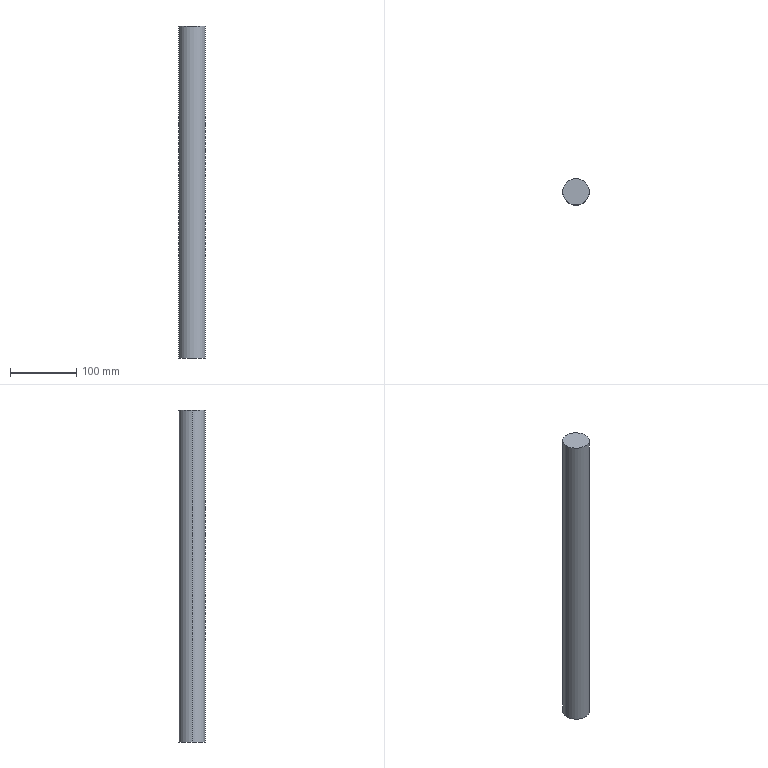Part | SolidWorks | features Extrusion 1 | 1 solid | 4 faces | box 40 x 40 x 500 mm | volume 628319 mm3 | cylinder 2 | plane 2 | commonest cylinder face diameters 40 x2
STEP:
#1=CARTESIAN_POINT('',(20.,0.,500.));
#2=VERTEX_POINT('',#1);
#3=CARTESIAN_POINT('',(-20.,0.,500.));
#4=VERTEX_POINT('',#3);
#5=CARTESIAN_POINT('',(0.,0.,500.));
#6=DIRECTION('',(0.,0.,1.));
#7=DIRECTION('',(1.,0.,0.));
#8=AXIS2_PLACEMENT_3D('',#5,#6,#7);
#9=CIRCLE('',#8,20.);
#10=EDGE_CURVE('',#2,#4,#9,.T.);
#11=ORIENTED_EDGE('',*,*,#10,.F.);
#12=CARTESIAN_POINT('',(20.,0.,0.));
#13=VERTEX_POINT('',#12);
#14=CARTESIAN_POINT('',(20.,0.,500.));
#15=DIRECTION('',(0.,0.,-1.));
#16=VECTOR('',#15,1000.);
#17=LINE('',#14,#16);
#18=EDGE_CURVE('',#2,#13,#17,.T.);
#19=ORIENTED_EDGE('',*,*,#18,.T.);
#20=CARTESIAN_POINT('',(-20.,0.,0.));
#21=VERTEX_POINT('',#20);
#22=CARTESIAN_POINT('',(0.,0.,0.));
#23=DIRECTION('',(0.,0.,1.));
#24=DIRECTION('',(1.,0.,0.));
#25=AXIS2_PLACEMENT_3D('',#22,#23,#24);
#26=CIRCLE('',#25,20.);
#27=EDGE_CURVE('',#13,#21,#26,.T.);
#28=ORIENTED_EDGE('',*,*,#27,.T.);
#29=CARTESIAN_POINT('',(-20.,0.,500.));
#30=DIRECTION('',(0.,0.,-1.));
#31=VECTOR('',#30,1000.);
#32=LINE('',#29,#31);
#33=EDGE_CURVE('',#4,#21,#32,.T.);
#34=ORIENTED_EDGE('',*,*,#33,.F.);
#35=EDGE_LOOP('',(#11,#19,#28,#34));
#36=FACE_OUTER_BOUND('',#35,.T.);
#37=CARTESIAN_POINT('',(0.,0.,500.));
#38=DIRECTION('',(0.,0.,-1.));
#39=DIRECTION('',(-1.,0.,0.));
#40=AXIS2_PLACEMENT_3D('',#37,#38,#39);
#41=CYLINDRICAL_SURFACE('',#40,20.);
#42=ADVANCED_FACE('',(#36),#41,.T.);
#43=ORIENTED_EDGE('',*,*,#18,.F.);
#44=CARTESIAN_POINT('',(0.,0.,500.));
#45=DIRECTION('',(0.,0.,1.));
#46=DIRECTION('',(1.,0.,0.));
#47=AXIS2_PLACEMENT_3D('',#44,#45,#46);
#48=CIRCLE('',#47,20.);
#49=EDGE_CURVE('',#4,#2,#48,.T.);
#50=ORIENTED_EDGE('',*,*,#49,.F.);
#51=ORIENTED_EDGE('',*,*,#33,.T.);
#52=CARTESIAN_POINT('',(0.,0.,0.));
#53=DIRECTION('',(0.,0.,1.));
#54=DIRECTION('',(1.,0.,0.));
#55=AXIS2_PLACEMENT_3D('',#52,#53,#54);
#56=CIRCLE('',#55,20.);
#57=EDGE_CURVE('',#21,#13,#56,.T.);
#58=ORIENTED_EDGE('',*,*,#57,.T.);
#59=EDGE_LOOP('',(#43,#50,#51,#58));
#60=FACE_OUTER_BOUND('',#59,.T.);
#61=CARTESIAN_POINT('',(0.,0.,500.));
#62=DIRECTION('',(0.,0.,-1.));
#63=DIRECTION('',(-1.,0.,0.));
#64=AXIS2_PLACEMENT_3D('',#61,#62,#63);
#65=CYLINDRICAL_SURFACE('',#64,20.);
#66=ADVANCED_FACE('',(#60),#65,.T.);
#67=ORIENTED_EDGE('',*,*,#49,.T.);
#68=ORIENTED_EDGE('',*,*,#10,.T.);
#69=EDGE_LOOP('',(#67,#68));
#70=FACE_OUTER_BOUND('',#69,.T.);
#71=CARTESIAN_POINT('',(0.,0.,500.));
#72=DIRECTION('',(0.,0.,1.));
#73=DIRECTION('',(1.,0.,0.));
#74=AXIS2_PLACEMENT_3D('',#71,#72,#73);
#75=PLANE('',#74);
#76=ADVANCED_FACE('',(#70),#75,.T.);
#77=ORIENTED_EDGE('',*,*,#57,.F.);
#78=ORIENTED_EDGE('',*,*,#27,.F.);
#79=EDGE_LOOP('',(#77,#78));
#80=FACE_OUTER_BOUND('',#79,.T.);
#81=CARTESIAN_POINT('',(0.,0.,0.));
#82=DIRECTION('',(0.,0.,1.));
#83=DIRECTION('',(1.,0.,0.));
#84=AXIS2_PLACEMENT_3D('',#81,#82,#83);
#85=PLANE('',#84);
#86=ADVANCED_FACE('',(#80),#85,.F.);
#87=CLOSED_SHELL('',(#42,#66,#76,#86));
#88=MANIFOLD_SOLID_BREP('',#87);
#89=CARTESIAN_POINT('',(0.,0.,0.));
#90=DIRECTION('',(0.,0.,1.));
#91=DIRECTION('',(1.,0.,0.));
#92=AXIS2_PLACEMENT_3D('',#89,#90,#91);
#93=(LENGTH_UNIT()NAMED_UNIT(*)SI_UNIT(.MILLI.,.METRE.));
#94=UNCERTAINTY_MEASURE_WITH_UNIT(LENGTH_MEASURE(0.00001),#93,'','');
#95=(NAMED_UNIT(*)PLANE_ANGLE_UNIT()SI_UNIT($,.RADIAN.));
#96=(NAMED_UNIT(*)SI_UNIT($,.STERADIAN.)SOLID_ANGLE_UNIT());
#97=(GEOMETRIC_REPRESENTATION_CONTEXT(3)GLOBAL_UNCERTAINTY_ASSIGNED_CONTEXT((#94))GLOBAL_UNIT_ASSIGNED_CONTEXT((#93,#95,#96))REPRESENTATION_CONTEXT('',''));
#98=ADVANCED_BREP_SHAPE_REPRESENTATION('',(#88,#92),#97);